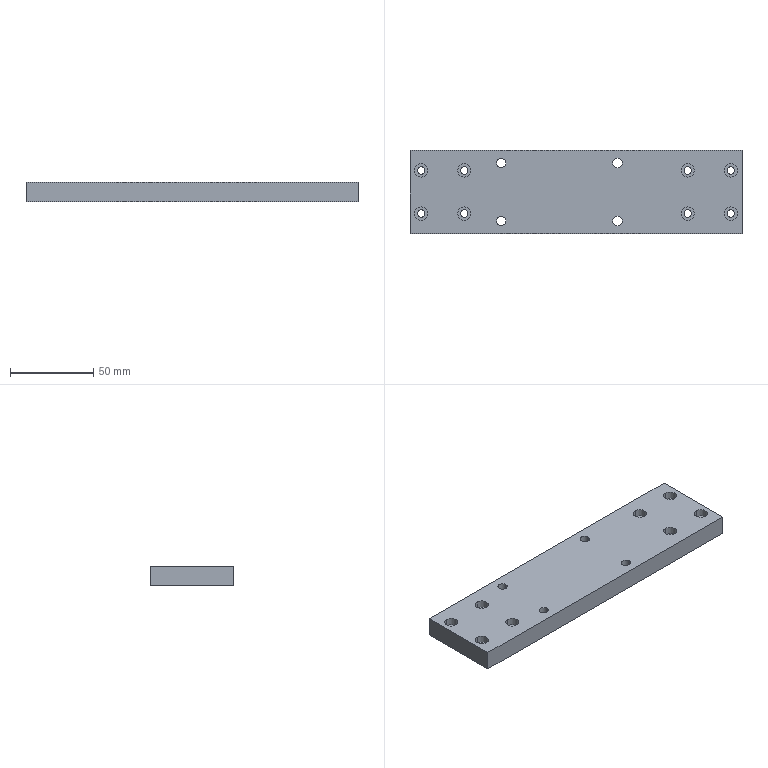Part | STEP file | X77-04101 | 1 solid | 54 faces | box 200 x 50 x 12 mm | volume 116026 mm3 | cylinder 40 | plane 14 | commonest cylinder face diameters 4.5 x16 8 x16 5.6 x8